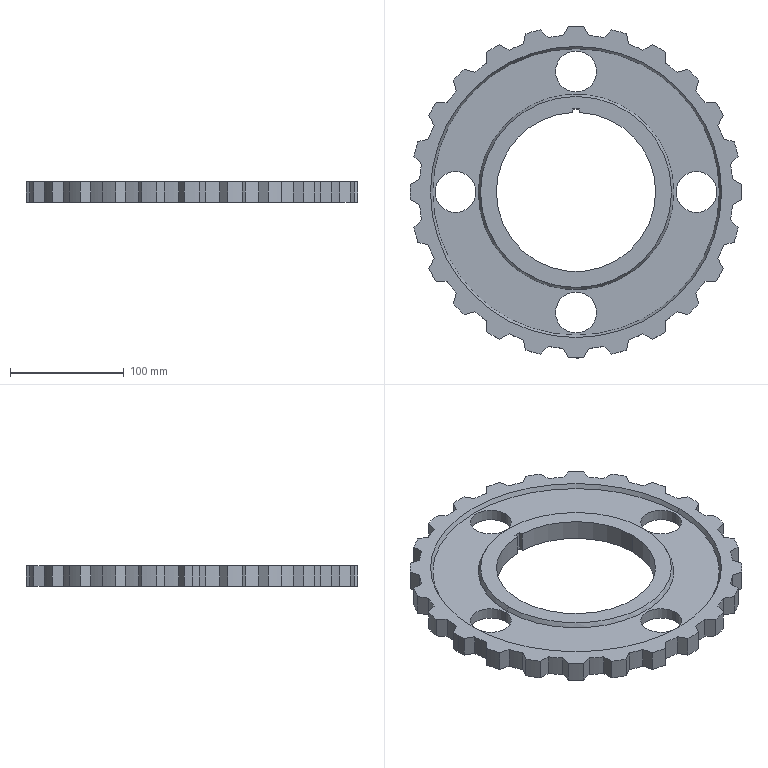Part | NX | features BREP 1 | 1 solid | 125 faces | box 292 x 292 x 18 mm | volume 597492 mm3 | cylinder 60 | plane 57 | cone 8 | commonest cylinder face diameters 292 x25 276 x24 36 x8 140 x3